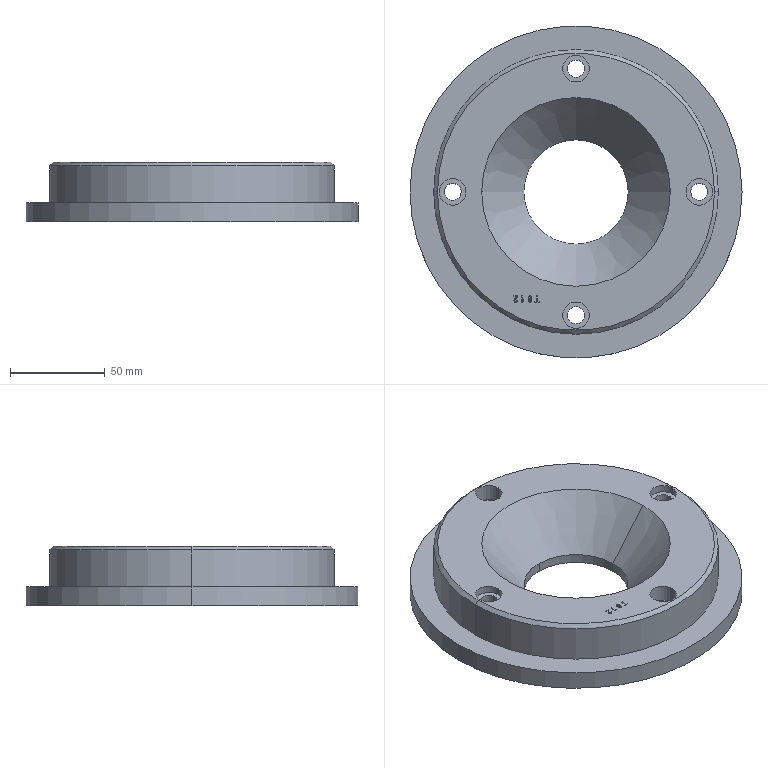Part | Creo | 1 solid | 111 faces | box 175 x 175 x 31.5 mm | volume 469696 mm3 | other 54 | plane 29 | cylinder 24 | cone 4 | commonest cylinder face diameters 9 x8 14 x8 55 x2 150 x2 175 x2 1.666 x1